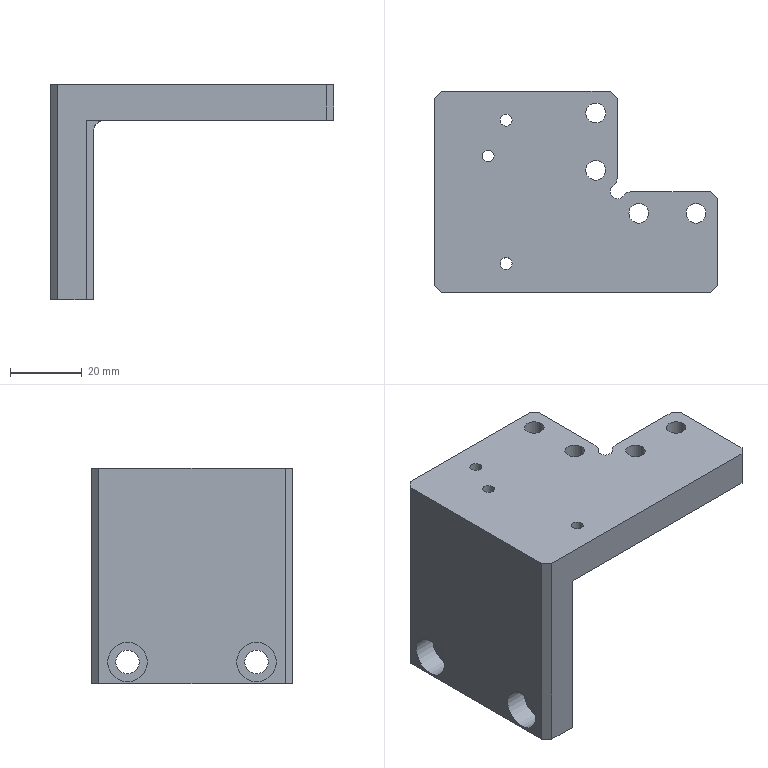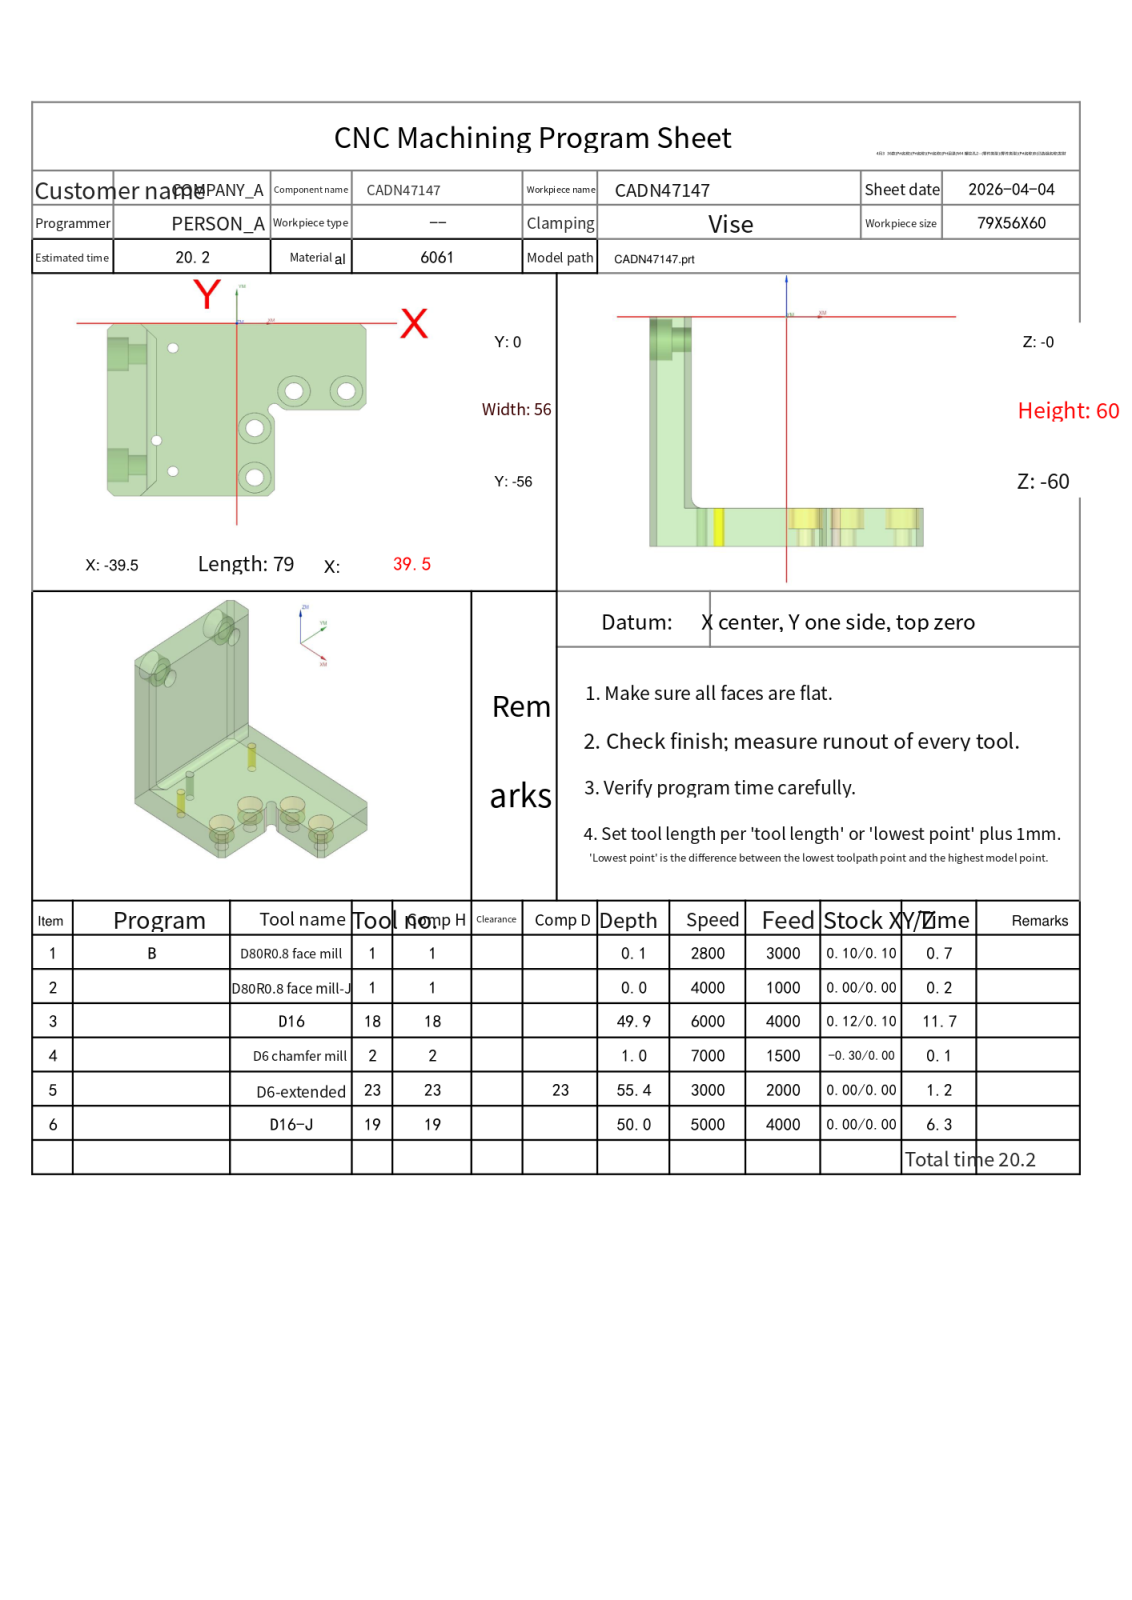NC program | NX | posted by the shop | part box 79 x 56 x 60 mm
Lines 110 to 1405 of 15895:
N3 T18 M06
(D16  D=16. R=0. H=18 ce=0.12 di=0.10)
G00 G90 G54 X-1.1 Y11.28 M03 S6000
G43 H18 Z14.5
M08
Z.701
G01 Z-.499 F4000.
G03 X10.1 Y.08 I11.2 J0.0
G01 X37.5
X37.557 Y.056
X39.557 Y-1.976
X39.58 Y-2.032
Y-26.
X39.557 Y-26.057
X37.556 Y-28.057
X37.499 Y-28.081
X15.495 Y-28.08
X15.117 Y-28.056
X14.247 Y-27.86
X14.218 Y-27.847
X13.495 Y-27.337
X12.839 Y-26.625
X12.085 Y-26.096
X11.211 Y-26.103
X10.436 Y-26.338
X9.782 Y-27.065
X9.565 Y-27.825
X9.608 Y-28.325
X9.784 Y-28.942
X10.303 Y-29.492
X10.704 Y-29.894
X10.927 Y-30.079
X10.945 Y-30.101
X11.47 Y-31.027
X11.48 Y-31.057
X11.58 Y-31.95
Y-54.
X11.557 Y-54.057
X9.557 Y-56.057
X9.5 Y-56.08
X-18.106
X-18.349 Y-56.294
X-18.437 Y-56.391
X-18.8 Y-56.843
X-19. Y-57.073
X-19.317 Y-57.412
X-21.009 Y-59.106
X-21.187 Y-59.3
X-21.54 Y-59.677
X-21.734 Y-59.871
X-23.701 Y-61.8
X-23.759 Y-61.863
X-23.815 Y-61.798
X-21.758 Y-59.742
X-21.568 Y-59.544
G03 X-19.38 Y-54. I-5.932 J5.544
G01 Y-53.984
Y-1.493
G03 X-19.589 Y-.168 I-8.446 J-.656
X-20.926 Y2.766 I-7.911 J-1.832
X-21.288 Y3.239 I-6.9 J-4.915
X-21.614 Y3.597 I-3.886 J-3.202
G01 X-23.815 Y5.798
X-23.795 Y5.818
X-23.738 Y5.882
X-23.682 Y5.819
X-22.702 Y4.839
X-21.68 Y3.819
X-21.485 Y3.622
X-21.01 Y3.105
X-20.164 Y2.258
X-19.315 Y1.41
X-18.997 Y1.069
X-18.197 Y.096
X-18.168 Y.08
X5.277
G02 X6.578 Y-.59 I-.001 J-1.6
G01 X13.622 Y-10.45
G03 X14.923 Y-11.12 I1.302 J.93
G01 X26.782
G02 X28.38 Y-12.718 I-.002 J-1.6
G01 Y-15.283
G02 X26.782 Y-16.88 I-1.6 J.002
G01 X18.928
G02 X18.077 Y-16.633 I.002 J1.6
G03 X12.085 Y-14.896 I-5.991 J-9.463
G01 X11.999
X9.504 Y-14.916
X7.179 Y-15.622
G03 X2.112 Y-18.845 I3.258 J-10.716
G01 X1.458 Y-19.572
G03 X-.988 Y-23.99 I8.324 J-7.493
G01 X-1.204 Y-24.75
G03 X-1.635 Y-27.825 I10.77 J-3.075
X-1.594 Y-28.78 I11.2 J0.0
G01 X-1.459 Y-30.359
X-.986 Y-32.016
G03 X.156 Y-34.664 I10.77 J3.075
G02 X.38 Y-35.477 I-1.377 J-.815
G01 Y-43.282
G02 X-1.218 Y-44.88 I-1.6 J.002
G01 X-6.582
G02 X-8.18 Y-43.282 I.002 J1.6
G01 Y-12.718
G02 X-6.582 Y-11.12 I1.6 J-.002
G01 X10.1
X10.6
G03 X21.8 Y.08 I0.0 J11.2
G01 Y11.28
Z.701
G00 Z3.
G01 X-1.1 F6000.
G00 Z.202
G01 Z-.998 F4000.
G03 X10.1 Y.08 I11.2 J0.0
G01 X37.5
X37.557 Y.056
X39.557 Y-1.976
X39.58 Y-2.032
Y-26.
X39.557 Y-26.057
X37.556 Y-28.057
X37.499 Y-28.081
X15.495 Y-28.08
X15.117 Y-28.056
X14.247 Y-27.86
X14.218 Y-27.847
X13.495 Y-27.337
X12.839 Y-26.625
X12.085 Y-26.096
X11.211 Y-26.103
X10.436 Y-26.338
X9.782 Y-27.065
X9.565 Y-27.825
X9.608 Y-28.325
X9.784 Y-28.942
X10.303 Y-29.492
X10.704 Y-29.894
X10.927 Y-30.079
X10.945 Y-30.101
X11.47 Y-31.027
X11.48 Y-31.057
X11.58 Y-31.95
Y-54.
X11.557 Y-54.057
X9.557 Y-56.057
X9.5 Y-56.08
X-17.351
X-18.106
X-18.349 Y-56.294
X-18.437 Y-56.391
X-18.687 Y-56.702
X-18.8 Y-56.843
X-18.892 Y-56.949
X-19. Y-57.073
X-19.317 Y-57.412
X-21.009 Y-59.106
X-21.54 Y-59.677
X-21.734 Y-59.871
X-23.701 Y-61.8
X-23.759 Y-61.863
X-23.815 Y-61.798
X-22.771 Y-60.755
X-21.758 Y-59.742
X-21.568 Y-59.544
G03 X-19.38 Y-54. I-5.932 J5.544
G01 Y-53.984
Y-1.493
G03 X-19.589 Y-.168 I-8.446 J-.656
X-20.926 Y2.766 I-7.911 J-1.832
X-21.288 Y3.239 I-6.9 J-4.915
X-21.454 Y3.43 I-3.886 J-3.202
X-21.758 Y3.742 I-3.756 J-3.36
G01 X-23.815 Y5.798
X-23.795 Y5.818
X-23.738 Y5.882
X-23.682 Y5.819
X-22.702 Y4.839
X-21.68 Y3.819
X-21.485 Y3.622
X-21.189 Y3.3
X-21.01 Y3.105
X-19.315 Y1.41
X-18.997 Y1.069
X-18.435 Y.389
X-18.197 Y.096
X-18.168 Y.08
X5.277
G02 X6.578 Y-.59 I-.001 J-1.6
G01 X13.622 Y-10.45
G03 X14.923 Y-11.12 I1.302 J.93
G01 X26.783
G02 X28.38 Y-12.717 I-.003 J-1.6
G01 Y-15.283
G02 X26.783 Y-16.88 I-1.6 J.003
G01 X18.928
G02 X18.077 Y-16.633 I.003 J1.6
G03 X12.085 Y-14.896 I-5.991 J-9.463
G01 X11.999
X9.504 Y-14.916
X7.179 Y-15.622
G03 X2.112 Y-18.845 I3.258 J-10.716
G01 X1.458 Y-19.572
G03 X-.988 Y-23.99 I8.324 J-7.493
G01 X-1.204 Y-24.75
G03 X-1.635 Y-27.825 I10.77 J-3.075
X-1.594 Y-28.78 I11.2 J0.0
G01 X-1.459 Y-30.359
X-.986 Y-32.016
G03 X.156 Y-34.664 I10.77 J3.075
G02 X.38 Y-35.477 I-1.377 J-.815
G01 Y-43.283
G02 X-1.218 Y-44.88 I-1.6 J.003
G01 X-6.583
G02 X-8.18 Y-43.283 I.003 J1.6
G01 Y-12.717
G02 X-6.583 Y-11.12 I1.6 J-.003
G01 X10.1
X10.6
G03 X21.8 Y.08 I0.0 J11.2
G01 Y11.28
Z.202
G00 Z2.501
G01 X-1.1 F6000.
G00 Z-.297
G01 Z-1.497 F4000.
G03 X10.1 Y.08 I11.2 J0.0
G01 X37.5
X37.557 Y.056
X39.557 Y-1.976
X39.58 Y-2.032
Y-26.
X39.557 Y-26.057
X37.556 Y-28.057
X37.499 Y-28.081
X15.495 Y-28.08
X15.117 Y-28.056
X14.247 Y-27.86
X14.218 Y-27.847
X13.495 Y-27.337
X12.839 Y-26.625
X12.085 Y-26.096
X11.211 Y-26.103
X10.436 Y-26.338
X9.782 Y-27.065
X9.565 Y-27.825
X9.608 Y-28.325
X9.784 Y-28.942
X10.303 Y-29.492
X10.704 Y-29.894
X10.927 Y-30.079
X10.945 Y-30.101
X11.47 Y-31.027
X11.48 Y-31.057
X11.58 Y-31.95
Y-54.
X11.557 Y-54.057
X9.557 Y-56.057
X9.5 Y-56.08
X-18.106
X-18.349 Y-56.294
X-18.437 Y-56.391
X-18.8 Y-56.843
X-19. Y-57.073
X-19.32 Y-57.415
X-21.009 Y-59.106
X-21.172 Y-59.284
X-21.54 Y-59.677
X-21.734 Y-59.871
X-23.701 Y-61.8
X-23.759 Y-61.863
X-23.815 Y-61.798
X-21.758 Y-59.742
X-21.568 Y-59.544
G03 X-19.38 Y-54. I-5.932 J5.544
G01 Y-53.984
Y-1.999
Y-1.493
G03 X-19.589 Y-.168 I-8.446 J-.656
X-20.926 Y2.766 I-7.911 J-1.832
X-21.288 Y3.239 I-6.9 J-4.915
X-21.614 Y3.597 I-3.886 J-3.202
G01 X-21.758 Y3.742
X-23.815 Y5.798
X-23.795 Y5.818
X-23.738 Y5.882
X-23.682 Y5.819
X-22.702 Y4.839
X-21.68 Y3.819
X-21.485 Y3.622
X-21.01 Y3.105
X-20.164 Y2.258
X-19.315 Y1.41
X-18.997 Y1.069
X-18.611 Y.601
X-18.435 Y.389
X-18.188 Y.091
X-18.168 Y.08
X-17.349
X5.277
G02 X6.578 Y-.59 I-.001 J-1.6
G01 X13.622 Y-10.45
G03 X14.923 Y-11.12 I1.302 J.93
G01 X26.783
G02 X28.38 Y-12.717 I-.003 J-1.6
G01 Y-15.283
G02 X26.783 Y-16.88 I-1.6 J.003
G01 X18.928
G02 X18.077 Y-16.633 I.003 J1.6
G03 X12.085 Y-14.896 I-5.992 J-9.463
G01 X11.999
X9.504 Y-14.916
X7.179 Y-15.622
G03 X2.112 Y-18.845 I3.258 J-10.716
G01 X1.458 Y-19.572
G03 X-.988 Y-23.99 I8.324 J-7.493
G01 X-1.204 Y-24.75
G03 X-1.635 Y-27.825 I10.77 J-3.075
X-1.594 Y-28.78 I11.2 J0.0
G01 X-1.459 Y-30.359
X-.986 Y-32.016
G03 X.157 Y-34.664 I10.77 J3.075
G02 X.38 Y-35.477 I-1.377 J-.815
G01 Y-43.283
G02 X-1.217 Y-44.88 I-1.6 J.003
G01 X-6.583
G02 X-8.18 Y-43.283 I.003 J1.6
G01 Y-12.717
G02 X-6.583 Y-11.12 I1.6 J-.003
G01 X10.1
X10.6
G03 X21.8 Y.08 I0.0 J11.2
G01 Y11.28
Z-.297
G00 Z2.002
G01 X-1.1 F6000.
G00 Z-.796
G01 Z-1.996 F4000.
G03 X10.1 Y.08 I11.2 J0.0
G01 X37.5
X37.557 Y.056
X39.557 Y-1.976
X39.58 Y-2.032
Y-26.
X39.557 Y-26.057
X37.556 Y-28.057
X37.499 Y-28.081
X15.495 Y-28.08
X15.117 Y-28.056
X14.247 Y-27.86
X14.218 Y-27.847
X13.495 Y-27.337
X12.839 Y-26.625
X12.085 Y-26.096
X11.211 Y-26.103
X10.436 Y-26.338
X9.782 Y-27.065
X9.565 Y-27.825
X9.608 Y-28.325
X9.784 Y-28.942
X10.303 Y-29.492
X10.704 Y-29.894
X10.927 Y-30.079
X10.945 Y-30.101
X11.47 Y-31.027
X11.48 Y-31.057
X11.58 Y-31.95
Y-54.
X11.557 Y-54.057
X9.557 Y-56.057
X9.5 Y-56.08
X-18.106
X-18.349 Y-56.294
X-18.437 Y-56.391
X-18.8 Y-56.843
X-19. Y-57.073
X-19.317 Y-57.412
X-21.009 Y-59.106
X-21.54 Y-59.677
X-21.734 Y-59.871
X-23.701 Y-61.8
X-23.759 Y-61.863
X-23.815 Y-61.798
X-21.758 Y-59.742
X-21.568 Y-59.544
G03 X-19.38 Y-54. I-5.932 J5.544
G01 Y-1.999
Y-1.493
G03 X-19.589 Y-.168 I-8.446 J-.656
X-20.926 Y2.766 I-7.911 J-1.832
X-21.288 Y3.239 I-6.9 J-4.915
X-21.758 Y3.742 I-3.909 J-3.181
G01 X-23.815 Y5.798
X-23.795 Y5.818
X-23.738 Y5.882
X-23.682 Y5.819
X-22.702 Y4.839
X-21.68 Y3.819
X-21.485 Y3.622
X-21.01 Y3.105
X-19.315 Y1.41
X-18.997 Y1.069
X-18.197 Y.096
X-18.168 Y.08
X5.277
G02 X6.578 Y-.59 I-.001 J-1.6
G01 X13.622 Y-10.45
G03 X14.923 Y-11.12 I1.302 J.93
G01 X26.783
G02 X28.38 Y-12.717 I-.003 J-1.6
G01 Y-15.283
G02 X26.783 Y-16.88 I-1.6 J.003
G01 X18.927
G02 X18.077 Y-16.634 I.003 J1.6
G03 X12.085 Y-14.896 I-5.992 J-9.462
G01 X11.999
X9.504 Y-14.916
X7.179 Y-15.622
G03 X2.112 Y-18.845 I3.258 J-10.716
G01 X1.458 Y-19.572
G03 X-.988 Y-23.99 I8.324 J-7.493
G01 X-1.204 Y-24.75
G03 X-1.635 Y-27.825 I10.77 J-3.075
X-1.594 Y-28.78 I11.2 J0.0
G01 X-1.459 Y-30.359
X-.986 Y-32.016
G03 X.157 Y-34.665 I10.77 J3.075
G02 X.38 Y-35.476 I-1.377 J-.815
G01 Y-43.283
G02 X-1.217 Y-44.88 I-1.6 J.003
G01 X-6.583
G02 X-8.18 Y-43.283 I.003 J1.6
G01 Y-12.717
G02 X-6.583 Y-11.12 I1.6 J-.003
G01 X10.1
X10.6
G03 X21.8 Y.08 I0.0 J11.2
G01 Y11.28
Z-.796
G00 Z1.503
G01 X-1.1 F6000.
G00 Z-1.295
G01 Z-2.495 F4000.
G03 X10.1 Y.08 I11.2 J0.0
G01 X37.5
X37.557 Y.056
X39.557 Y-1.976
X39.58 Y-2.032
Y-26.
X39.557 Y-26.057
X37.556 Y-28.057
X37.499 Y-28.081
X15.495 Y-28.08
X15.117 Y-28.056
X14.247 Y-27.86
X14.218 Y-27.847
X13.495 Y-27.337
X12.839 Y-26.625
X12.085 Y-26.096
X11.211 Y-26.103
X10.436 Y-26.338
X9.782 Y-27.065
X9.565 Y-27.825
X9.608 Y-28.325
X9.784 Y-28.942
X10.303 Y-29.492
X10.704 Y-29.894
X10.927 Y-30.079
X10.945 Y-30.101
X11.47 Y-31.027
X11.48 Y-31.057
X11.58 Y-31.95
Y-54.
X11.557 Y-54.057
X9.557 Y-56.057
X9.5 Y-56.08
X-18.106
X-18.349 Y-56.294
X-18.437 Y-56.391
X-18.8 Y-56.843
X-19. Y-57.073
X-19.317 Y-57.412
X-21.009 Y-59.106
X-21.54 Y-59.677
X-21.734 Y-59.871
X-23.701 Y-61.8
X-23.759 Y-61.863
X-23.815 Y-61.798
X-21.758 Y-59.742
X-21.568 Y-59.544
G03 X-19.38 Y-54. I-5.932 J5.544
G01 Y-1.999
Y-1.493
G03 X-19.589 Y-.168 I-8.446 J-.656
X-20.926 Y2.766 I-7.911 J-1.832
X-21.288 Y3.239 I-6.9 J-4.915
X-21.614 Y3.597 I-3.886 J-3.202
G01 X-21.758 Y3.742
X-23.815 Y5.798
X-23.795 Y5.818
X-23.738 Y5.882
X-23.682 Y5.819
X-22.702 Y4.839
X-21.68 Y3.819
X-21.485 Y3.622
X-21.01 Y3.105
X-19.315 Y1.41
X-19.163 Y1.247
X-18.997 Y1.069
X-18.435 Y.389
X-18.197 Y.096
X-18.168 Y.08
X5.277
G02 X6.578 Y-.59 I-.001 J-1.6
G01 X13.622 Y-10.45
G03 X14.923 Y-11.12 I1.302 J.93
G01 X26.783
G02 X28.38 Y-12.717 I-.003 J-1.6
G01 Y-15.283
G02 X26.783 Y-16.88 I-1.6 J.003
G01 X18.927
G02 X18.077 Y-16.634 I.003 J1.6
G03 X12.085 Y-14.896 I-5.992 J-9.462
G01 X11.999
X9.504 Y-14.916
X7.179 Y-15.622
G03 X2.112 Y-18.845 I3.258 J-10.716
G01 X1.458 Y-19.572
G03 X-.988 Y-23.99 I8.324 J-7.493
G01 X-1.204 Y-24.75
G03 X-1.635 Y-27.825 I10.77 J-3.075
X-1.594 Y-28.78 I11.2 J0.0
G01 X-1.459 Y-30.359
X-.986 Y-32.016
G03 X.157 Y-34.665 I10.77 J3.075
G02 X.38 Y-35.476 I-1.377 J-.815
G01 Y-43.283
G02 X-1.217 Y-44.88 I-1.6 J.003
G01 X-6.583
G02 X-8.18 Y-43.283 I.003 J1.6
G01 Y-12.717
G02 X-6.583 Y-11.12 I1.6 J-.003
G01 X10.1
X10.6
G03 X21.8 Y.08 I0.0 J11.2
G01 Y11.28
Z-1.295
G00 Z1.004
G01 X-1.1 F6000.
G00 Z-1.794
G01 Z-2.994 F4000.
G03 X10.1 Y.08 I11.2 J0.0
G01 X37.5
X37.557 Y.056
X39.557 Y-1.976
X39.58 Y-2.032
Y-26.
X39.557 Y-26.057
X37.556 Y-28.057
X37.499 Y-28.081
X15.495 Y-28.08
X15.117 Y-28.056
X14.247 Y-27.86
X14.218 Y-27.847
X13.495 Y-27.337
X12.839 Y-26.625
X12.085 Y-26.096
X11.211 Y-26.103
X10.436 Y-26.338
X9.782 Y-27.065
X9.565 Y-27.825
X9.608 Y-28.325
X9.784 Y-28.942
X10.303 Y-29.492
X10.704 Y-29.894
X10.927 Y-30.079
X10.945 Y-30.101
X11.47 Y-31.027
X11.48 Y-31.057
X11.58 Y-31.95
Y-54.
X11.557 Y-54.057
X9.557 Y-56.057
X9.5 Y-56.08
X-17.351
X-18.106
X-18.349 Y-56.294
X-18.437 Y-56.391
X-18.8 Y-56.843
X-19. Y-57.073
X-19.317 Y-57.412
X-21.009 Y-59.106
X-21.187 Y-59.3
X-21.54 Y-59.677
X-21.734 Y-59.871
X-23.701 Y-61.8
X-23.759 Y-61.863
X-23.815 Y-61.798
X-21.758 Y-59.742
X-21.568 Y-59.544
G03 X-19.38 Y-54. I-5.932 J5.544
G01 Y-1.999
Y-1.493
G03 X-19.589 Y-.168 I-8.446 J-.656
X-20.926 Y2.766 I-7.911 J-1.832
X-21.288 Y3.239 I-6.9 J-4.915
X-21.614 Y3.597 I-3.886 J-3.202
G01 X-21.758 Y3.742
X-23.815 Y5.798
X-23.795 Y5.818
X-23.738 Y5.882
X-23.682 Y5.819
X-22.702 Y4.839
X-21.68 Y3.819
X-21.485 Y3.622
X-21.189 Y3.3
X-21.01 Y3.105
X-19.315 Y1.41
X-18.997 Y1.069
X-18.435 Y.389
X-18.197 Y.096
X-18.168 Y.08
X5.277
G02 X6.578 Y-.59 I-.001 J-1.6
G01 X13.622 Y-10.45
G03 X14.923 Y-11.12 I1.302 J.93
G01 X26.783
G02 X28.38 Y-12.717 I-.003 J-1.6
G01 Y-15.284
G02 X26.783 Y-16.88 I-1.6 J.003
G01 X18.927
G02 X18.077 Y-16.634 I.003 J1.6
G03 X12.085 Y-14.896 I-5.992 J-9.462
G01 X11.999
X9.504 Y-14.916
X7.179 Y-15.622
G03 X2.112 Y-18.845 I3.258 J-10.716
G01 X1.458 Y-19.572
G03 X-.988 Y-23.99 I8.324 J-7.493
G01 X-1.204 Y-24.75
G03 X-1.635 Y-27.825 I10.77 J-3.075
X-1.594 Y-28.78 I11.2 J0.0
G01 X-1.459 Y-30.359
X-.986 Y-32.016
G03 X.157 Y-34.665 I10.77 J3.075
G02 X.38 Y-35.476 I-1.377 J-.815
G01 Y-43.283
G02 X-1.217 Y-44.88 I-1.6 J.003
G01 X-6.583
G02 X-8.18 Y-43.283 I.003 J1.6
G01 Y-12.717
G02 X-6.583 Y-11.12 I1.6 J-.003
G01 X10.1
X10.6
G03 X21.8 Y.08 I0.0 J11.2
G01 Y11.28
Z-1.794
G00 Z.505
G01 X-1.1 F6000.
G00 Z-2.293
G01 Z-3.493 F4000.
G03 X10.1 Y.08 I11.2 J0.0
G01 X37.5
X37.557 Y.056
X39.557 Y-1.976
X39.58 Y-2.032
Y-26.
X39.557 Y-26.057
X37.556 Y-28.057
X37.499 Y-28.081
X15.495 Y-28.08
X15.117 Y-28.056
X14.247 Y-27.86
X14.218 Y-27.847
X13.495 Y-27.337
X12.839 Y-26.625
X12.085 Y-26.096
X11.211 Y-26.103
X10.436 Y-26.338
X9.782 Y-27.065
X9.565 Y-27.825
X9.608 Y-28.325
X9.784 Y-28.942
X10.303 Y-29.492
X10.704 Y-29.894
X10.927 Y-30.079
X10.945 Y-30.101
X11.47 Y-31.027
X11.48 Y-31.057
X11.58 Y-31.95
Y-54.
X11.557 Y-54.057
X9.557 Y-56.057
X9.5 Y-56.08
X-18.106
X-18.227 Y-56.187
X-18.349 Y-56.294
X-18.437 Y-56.391
X-18.548 Y-56.529
X-18.8 Y-56.843
X-19. Y-57.073
X-19.317 Y-57.412
X-21.009 Y-59.106
X-21.54 Y-59.677
X-21.734 Y-59.871
X-23.701 Y-61.8
X-23.759 Y-61.863
X-23.815 Y-61.798
X-21.758 Y-59.742
X-21.568 Y-59.544
G03 X-19.38 Y-54. I-5.932 J5.544
G01 Y-1.998
Y-1.493
G03 X-19.589 Y-.168 I-8.446 J-.656
X-20.926 Y2.766 I-7.911 J-1.832
X-21.288 Y3.239 I-6.9 J-4.915
X-21.614 Y3.597 I-3.886 J-3.202
G01 X-21.758 Y3.742
X-23.815 Y5.798
X-23.795 Y5.818
X-23.738 Y5.882
X-23.682 Y5.819
X-22.702 Y4.839
X-21.68 Y3.819
X-21.485 Y3.622
X-21.189 Y3.3
X-21.01 Y3.105
X-19.315 Y1.41
X-18.997 Y1.069
X-18.435 Y.389
X-18.197 Y.096
X-18.168 Y.08
X5.277
G02 X6.578 Y-.59 I-.001 J-1.6
G01 X13.622 Y-10.45
G03 X14.923 Y-11.12 I1.302 J.93
G01 X26.784
G02 X28.38 Y-12.716 I-.004 J-1.6
G01 Y-15.284
G02 X26.784 Y-16.88 I-1.6 J.004
G01 X18.927
G02 X18.078 Y-16.634 I.004 J1.6
G03 X12.085 Y-14.896 I-5.992 J-9.462
G01 X11.999
X9.504 Y-14.916
X7.179 Y-15.622
G03 X2.112 Y-18.845 I3.258 J-10.716
G01 X1.458 Y-19.572
G03 X-.988 Y-23.99 I8.324 J-7.493
G01 X-1.204 Y-24.75
G03 X-1.635 Y-27.825 I10.77 J-3.075
X-1.594 Y-28.78 I11.2 J0.0
G01 X-1.459 Y-30.359
X-.986 Y-32.016
G03 X.157 Y-34.665 I10.77 J3.075
G02 X.38 Y-35.476 I-1.377 J-.814
G01 Y-43.284
G02 X-1.217 Y-44.88 I-1.6 J.003
G01 X-6.584
G02 X-8.18 Y-43.284 I.004 J1.6
G01 Y-12.716
G02 X-6.584 Y-11.12 I1.6 J-.004
G01 X10.1
X10.6
G03 X21.8 Y.08 I0.0 J11.2
G01 Y11.28
Z-2.293
G00 Z.006
G01 X-1.1 F6000.
G00 Z-2.792
G01 Z-3.992 F4000.
G03 X10.1 Y.08 I11.2 J0.0
G01 X37.5
X37.557 Y.056
X39.557 Y-1.976
X39.58 Y-2.032
Y-26.
X39.557 Y-26.057
X37.556 Y-28.057
X37.499 Y-28.081
X15.495 Y-28.08
X15.117 Y-28.056
X14.247 Y-27.86
X14.218 Y-27.847
X13.495 Y-27.337
X12.839 Y-26.625
X12.085 Y-26.096
X11.211 Y-26.103
X10.436 Y-26.338
X9.782 Y-27.065
X9.565 Y-27.825
X9.608 Y-28.325
X9.784 Y-28.942
X10.303 Y-29.492
X10.704 Y-29.894
X10.927 Y-30.079
X10.945 Y-30.101
X11.47 Y-31.027
X11.48 Y-31.057
X11.58 Y-31.95
Y-54.
X11.557 Y-54.057
X9.557 Y-56.057
X9.5 Y-56.08
X-18.106
X-18.349 Y-56.294
X-18.437 Y-56.391
X-18.8 Y-56.843
X-19. Y-57.073
X-19.157 Y-57.241
X-19.317 Y-57.412
X-21.035 Y-59.135
X-21.54 Y-59.677
X-21.734 Y-59.871
X-23.701 Y-61.8
X-23.759 Y-61.863
X-23.815 Y-61.798
X-21.758 Y-59.742
X-21.568 Y-59.544
G03 X-19.38 Y-54. I-5.932 J5.544
G01 Y-1.998
Y-1.493
G03 X-19.589 Y-.168 I-8.446 J-.656
X-20.926 Y2.766 I-7.911 J-1.832
X-21.288 Y3.239 I-6.9 J-4.915
X-21.614 Y3.597 I-3.886 J-3.202
G01 X-21.758 Y3.742
X-23.815 Y5.798
X-23.795 Y5.818
X-23.738 Y5.882
X-23.682 Y5.819
X-22.702 Y4.839
X-21.68 Y3.819
X-21.485 Y3.622
X-21.189 Y3.3
X-21.01 Y3.105
X-19.315 Y1.41
X-19.157 Y1.241
X-18.997 Y1.069
X-18.611 Y.601
X-18.435 Y.389
X-18.197 Y.096
X-18.168 Y.08
X5.277
G02 X6.578 Y-.59 I-.001 J-1.6
G01 X13.622 Y-10.45
G03 X14.923 Y-11.12 I1.302 J.93
G01 X26.784
G02 X28.38 Y-12.716 I-.004 J-1.6
G01 Y-15.284
G02 X26.784 Y-16.88 I-1.6 J.004
G01 X18.927
G02 X18.078 Y-16.634 I.004 J1.6
G03 X12.085 Y-14.896 I-5.992 J-9.462
G01 X11.999
X9.504 Y-14.916
X7.179 Y-15.622
G03 X2.112 Y-18.845 I3.258 J-10.716
G01 X1.458 Y-19.572
G03 X-.988 Y-23.99 I8.324 J-7.493
G01 X-1.204 Y-24.75
G03 X-1.635 Y-27.825 I10.77 J-3.075
X-1.594 Y-28.78 I11.2 J0.0
G01 X-1.459 Y-30.359
X-.986 Y-32.016
G03 X.157 Y-34.665 I10.77 J3.075
G02 X.38 Y-35.476 I-1.377 J-.814
G01 Y-43.284
G02 X-1.217 Y-44.88 I-1.6 J.004
G01 X-6.584
G02 X-8.18 Y-43.284 I.004 J1.6
G01 Y-12.716
G02 X-6.584 Y-11.12 I1.6 J-.004
G01 X10.1
X10.6
G03 X21.8 Y.08 I0.0 J11.2
G01 Y11.28
Z-2.792
G00 Z-.493
G01 X-1.1 F6000.
G00 Z-3.291
G01 Z-4.491 F4000.
G03 X10.1 Y.08 I11.2 J0.0
G01 X37.5
X37.557 Y.056
X39.557 Y-1.976
X39.58 Y-2.032
Y-26.
X39.557 Y-26.057
X37.556 Y-28.057
X37.499 Y-28.081
X15.495 Y-28.08
X15.117 Y-28.056
X14.247 Y-27.86
X14.218 Y-27.847
X13.495 Y-27.337
X12.839 Y-26.625
X12.085 Y-26.096
X11.211 Y-26.103
X10.436 Y-26.338
X9.782 Y-27.065
X9.565 Y-27.825
X9.608 Y-28.325
X9.784 Y-28.942
X10.303 Y-29.492
X10.704 Y-29.894
X10.927 Y-30.079
X10.945 Y-30.101
X11.47 Y-31.027
X11.48 Y-31.057
X11.58 Y-31.95
Y-54.
X11.557 Y-54.057
X9.557 Y-56.057
X9.5 Y-56.08
X-18.106
X-18.218 Y-56.179
X-18.349 Y-56.294
X-18.437 Y-56.391
X-18.617 Y-56.616
X-18.8 Y-56.843
X-19. Y-57.073
X-19.317 Y-57.412
X-21.009 Y-59.106
X-21.54 Y-59.677
X-21.734 Y-59.871
X-23.701 Y-61.8
X-23.759 Y-61.863
X-23.815 Y-61.798
X-21.758 Y-59.742
X-21.568 Y-59.544
G03 X-19.38 Y-54. I-5.932 J5.544
G01 Y-1.998
Y-1.493
X-19.39 Y-1.377
G03 X-19.589 Y-.168 I-8.436 J-.772
X-20.926 Y2.766 I-7.911 J-1.832
X-21.288 Y3.239 I-6.9 J-4.915
X-21.614 Y3.597 I-3.886 J-3.202
G01 X-21.758 Y3.742
X-23.815 Y5.798
X-23.795 Y5.818
X-23.738 Y5.882
X-23.682 Y5.819
X-22.702 Y4.839
X-21.68 Y3.819
X-21.485 Y3.622
X-21.189 Y3.3
X-21.01 Y3.105
X-19.315 Y1.41
X-18.997 Y1.069
X-18.197 Y.096
X-18.168 Y.08
X5.277
G02 X6.578 Y-.59 I-.001 J-1.6
G01 X13.622 Y-10.45
G03 X14.923 Y-11.12 I1.302 J.93
G01 X26.784
G02 X28.38 Y-12.716 I-.004 J-1.6
G01 Y-15.284
G02 X26.784 Y-16.88 I-1.6 J.004
G01 X18.926
G02 X18.078 Y-16.634 I.004 J1.6
G03 X12.085 Y-14.896 I-5.992 J-9.462
G01 X11.999
X9.504 Y-14.916
X7.179 Y-15.622
G03 X2.112 Y-18.845 I3.258 J-10.716
G01 X1.458 Y-19.572
G03 X-.988 Y-23.99 I8.324 J-7.493
G01 X-1.204 Y-24.75
G03 X-1.635 Y-27.825 I10.77 J-3.075
X-1.594 Y-28.78 I11.2 J0.0
G01 X-1.459 Y-30.359
X-.986 Y-32.016
G03 X.157 Y-34.665 I10.77 J3.075
G02 X.38 Y-35.476 I-1.377 J-.814
G01 Y-43.284
G02 X-1.216 Y-44.88 I-1.6 J.004
G01 X-6.584
G02 X-8.18 Y-43.284 I.004 J1.6
G01 Y-12.716
G02 X-6.584 Y-11.12 I1.6 J-.004
G01 X10.1
X10.6
G03 X21.8 Y.08 I0.0 J11.2
G01 Y11.28
Z-3.291
G00 Z-.992
G01 X-1.1 F6000.
G00 Z-3.79
G01 Z-4.99 F4000.
G03 X10.1 Y.08 I11.2 J0.0
G01 X37.5
X37.557 Y.056
X39.557 Y-1.976
X39.58 Y-2.032
Y-26.
X39.557 Y-26.057
X37.556 Y-28.057
X37.499 Y-28.081
X15.495 Y-28.08
X15.117 Y-28.056
X14.247 Y-27.86
X14.218 Y-27.847
X13.495 Y-27.337
X12.839 Y-26.625
X12.085 Y-26.096
X11.211 Y-26.103
X10.436 Y-26.338
X9.782 Y-27.065
X9.565 Y-27.825
X9.608 Y-28.325
X9.784 Y-28.942
X10.303 Y-29.492
X10.704 Y-29.894
X10.927 Y-30.079
X10.945 Y-30.101
X11.47 Y-31.027
X11.48 Y-31.057
X11.58 Y-31.95
Y-54.
X11.557 Y-54.057
X9.557 Y-56.057
X9.5 Y-56.08
X-18.106
X-18.349 Y-56.294
X-18.437 Y-56.391
X-18.8 Y-56.843
X-19. Y-57.073
X-19.157 Y-57.241
X-19.317 Y-57.412
X-21.009 Y-59.106
X-21.187 Y-59.3
X-21.54 Y-59.677
X-21.734 Y-59.871
X-23.701 Y-61.8
X-23.759 Y-61.863
X-23.815 Y-61.798
X-21.758 Y-59.742
X-21.568 Y-59.544
G03 X-19.38 Y-54. I-5.932 J5.544
G01 Y-1.998
Y-1.493
G03 X-19.589 Y-.168 I-8.446 J-.656
X-20.926 Y2.766 I-7.911 J-1.832
X-21.337 Y3.297 I-6.899 J-4.917
X-21.758 Y3.742 I-3.863 J-3.237
G01 X-23.815 Y5.798
X-23.795 Y5.818
X-23.738 Y5.882
X-23.682 Y5.819
X-22.702 Y4.839
X-21.68 Y3.819
X-21.485 Y3.622
X-21.01 Y3.105
X-19.315 Y1.41
X-19.157 Y1.241
X-18.997 Y1.069
X-18.435 Y.389
X-18.197 Y.096
X-18.168 Y.08
X5.277
G02 X6.578 Y-.59 I-.001 J-1.6
G01 X13.622 Y-10.45
G03 X14.923 Y-11.12 I1.302 J.93
G01 X26.784
G02 X28.38 Y-12.716 I-.004 J-1.6
G01 Y-15.284
G02 X26.784 Y-16.88 I-1.6 J.004
G01 X18.926
G02 X18.078 Y-16.634 I.004 J1.6
G03 X12.085 Y-14.896 I-5.993 J-9.462
G01 X11.999
X9.504 Y-14.916
X7.179 Y-15.622
G03 X2.112 Y-18.845 I3.258 J-10.716
G01 X1.458 Y-19.572
G03 X-.988 Y-23.99 I8.324 J-7.493
G01 X-1.204 Y-24.75
G03 X-1.635 Y-27.825 I10.77 J-3.075
X-1.594 Y-28.78 I11.2 J0.0
G01 X-1.459 Y-30.359
X-.986 Y-32.016
G03 X.157 Y-34.665 I10.77 J3.075
G02 X.38 Y-35.475 I-1.377 J-.814
G01 Y-43.284
G02 X-1.216 Y-44.88 I-1.6 J.004
G01 X-6.584
G02 X-8.18 Y-43.284 I.004 J1.6
G01 Y-12.716
G02 X-6.584 Y-11.12 I1.6 J-.004
G01 X10.1
X10.6
G03 X21.8 Y.08 I0.0 J11.2
G01 Y11.28
Z-3.79
G00 Z-1.491
G01 X-1.1 F6000.
G00 Z-4.289
G01 Z-5.489 F4000.
G03 X10.1 Y.08 I11.2 J0.0
G01 X37.5
X37.557 Y.056
X39.557 Y-1.976
X39.58 Y-2.032
Y-26.
X39.557 Y-26.057
X37.556 Y-28.057
X37.499 Y-28.081
X15.495 Y-28.08
X15.117 Y-28.056
X14.247 Y-27.86
X14.218 Y-27.847
X13.495 Y-27.337
X12.839 Y-26.625
X12.085 Y-26.096
X11.211 Y-26.103
X10.436 Y-26.338
X9.782 Y-27.065
X9.565 Y-27.825
X9.608 Y-28.325
X9.784 Y-28.942
X10.303 Y-29.492
X10.704 Y-29.894
X10.927 Y-30.079
X10.945 Y-30.101
X11.47 Y-31.027
X11.48 Y-31.057
X11.58 Y-31.95
Y-54.
X11.557 Y-54.057
X9.557 Y-56.057
X9.5 Y-56.08
X-18.106
X-18.227 Y-56.187
X-18.349 Y-56.294
X-18.437 Y-56.391
X-18.8 Y-56.843
X-19. Y-57.073
X-19.317 Y-57.412
X-21.009 Y-59.106
X-21.187 Y-59.3
X-21.54 Y-59.677
X-21.734 Y-59.871
X-23.701 Y-61.8
X-23.759 Y-61.863
X-23.815 Y-61.798
X-21.758 Y-59.742
X-21.568 Y-59.544
G03 X-19.38 Y-54. I-5.932 J5.544
G01 Y-1.998
Y-1.493
G03 X-19.589 Y-.168 I-8.446 J-.656
X-20.926 Y2.766 I-7.911 J-1.832
X-21.288 Y3.239 I-6.9 J-4.915
X-21.614 Y3.597 I-3.886 J-3.202
G01 X-21.758 Y3.742
X-23.815 Y5.798
X-23.795 Y5.818
X-23.738 Y5.882
X-23.682 Y5.819
X-22.702 Y4.839
X-21.68 Y3.819
X-21.485 Y3.622
X-21.01 Y3.105
X-19.315 Y1.41
X-18.997 Y1.069
X-18.197 Y.096
X-18.168 Y.08
X5.277
G02 X6.578 Y-.59 I-.001 J-1.6
G01 X13.622 Y-10.45
G03 X14.923 Y-11.12 I1.302 J.93
G01 X26.784
G02 X28.38 Y-12.716 I-.004 J-1.6
G01 Y-15.284
G02 X26.784 Y-16.88 I-1.6 J.004
G01 X18.926
G02 X18.078 Y-16.634 I.004 J1.6
G03 X12.085 Y-14.896 I-5.993 J-9.462
G01 X11.999
X9.504 Y-14.916
X7.179 Y-15.622
G03 X2.112 Y-18.845 I3.258 J-10.716
G01 X1.458 Y-19.572
G03 X-.988 Y-23.99 I8.324 J-7.493
G01 X-1.204 Y-24.75
G03 X-1.635 Y-27.825 I10.77 J-3.075
X-1.594 Y-28.78 I11.2 J0.0
G01 X-1.459 Y-30.359
X-.986 Y-32.016
G03 X.157 Y-34.666 I10.77 J3.075
G02 X.38 Y-35.475 I-1.378 J-.814
G01 Y-43.284
G02 X-1.216 Y-44.88 I-1.6 J.004
G01 X-6.584
G02 X-8.18 Y-43.284 I.004 J1.6
G01 Y-12.716
G02 X-6.584 Y-11.12 I1.6 J-.004
G01 X10.1
X10.6
G03 X21.8 Y.08 I0.0 J11.2
G01 Y11.28
Z-4.289
G00 Z-1.99
G01 X-1.1 F6000.
G00 Z-4.788
G01 Z-5.988 F4000.
G03 X10.1 Y.08 I11.2 J0.0
G01 X37.5
X37.557 Y.056
X39.557 Y-1.976
X39.58 Y-2.032
Y-26.
X39.557 Y-26.057
X37.556 Y-28.057
X37.499 Y-28.081
X15.495 Y-28.08
X15.117 Y-28.056
X14.247 Y-27.86
X14.218 Y-27.847
X13.495 Y-27.337
X12.839 Y-26.625
X12.085 Y-26.096
X11.211 Y-26.103
X10.436 Y-26.338
X9.782 Y-27.065
X9.565 Y-27.825
X9.608 Y-28.325
X9.784 Y-28.942
X10.303 Y-29.492
X10.704 Y-29.894
X10.927 Y-30.079
X10.945 Y-30.101
X11.47 Y-31.027
X11.48 Y-31.057
X11.58 Y-31.95
Y-54.
X11.557 Y-54.057
X9.557 Y-56.057
X9.5 Y-56.08
X-18.106
X-18.349 Y-56.294
X-18.437 Y-56.391
X-18.8 Y-56.843
X-19. Y-57.073
X-19.317 Y-57.412
X-21.009 Y-59.106
X-21.187 Y-59.3
X-21.54 Y-59.677
X-21.734 Y-59.871
X-23.701 Y-61.8
X-23.759 Y-61.863
X-23.815 Y-61.798
X-21.758 Y-59.742
X-21.568 Y-59.544
G03 X-19.38 Y-54. I-5.932 J5.544
G01 Y-1.998
Y-1.493
G03 X-19.597 Y-.137 I-8.447 J-.654
X-20.926 Y2.766 I-7.903 J-1.863
X-21.288 Y3.239 I-6.9 J-4.915
X-21.614 Y3.597 I-3.886 J-3.202
G01 X-21.758 Y3.742
X-22.758 Y4.742
X-23.815 Y5.798
X-23.795 Y5.818
X-23.738 Y5.882
X-23.682 Y5.819
X-22.702 Y4.839
X-21.68 Y3.819
X-21.485 Y3.622
X-21.189 Y3.3
X-21.01 Y3.105
X-19.315 Y1.41
X-18.997 Y1.069
X-18.435 Y.389
X-18.197 Y.096
X-18.168 Y.08
X5.277
G02 X6.578 Y-.59 I-.001 J-1.6
G01 X13.622 Y-10.45
G03 X14.923 Y-11.12 I1.302 J.93
G01 X26.784
G02 X28.38 Y-12.716 I-.004 J-1.6
G01 Y-15.285
G02 X26.784 Y-16.88 I-1.6 J.004
G01 X18.926
G02 X18.078 Y-16.634 I.004 J1.6
G03 X12.085 Y-14.896 I-5.993 J-9.462
G01 X11.999
X9.504 Y-14.916
X7.179 Y-15.622
G03 X2.112 Y-18.845 I3.258 J-10.716
G01 X1.458 Y-19.572